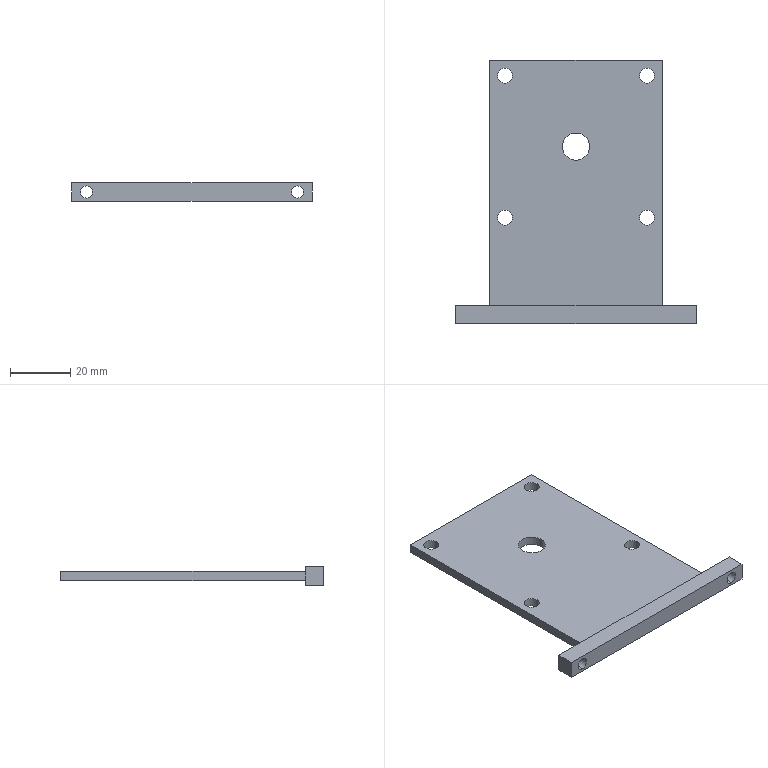Part | STEP file | Motor mounting plate | 1 solid | 29 faces | box 80 x 87.326 x 6 mm | volume 16246 mm3 | cylinder 14 | plane 11 | cone 4 | commonest cylinder face diameters 5 x8 4 x4 9 x2
STEP:
#1=CARTESIAN_POINT('',(-35.,-52.776,-0.5));
#2=VERTEX_POINT('',#1);
#3=CARTESIAN_POINT('',(-35.,-52.776,3.5));
#4=VERTEX_POINT('',#3);
#5=CARTESIAN_POINT('',(-35.,-52.776,1.5));
#6=DIRECTION('',(0.,1.,0.));
#7=DIRECTION('',(0.,0.,1.));
#8=AXIS2_PLACEMENT_3D('',#5,#6,#7);
#9=CIRCLE('',#8,2.);
#10=EDGE_CURVE('',#2,#4,#9,.T.);
#11=ORIENTED_EDGE('',*,*,#10,.F.);
#12=CARTESIAN_POINT('',(-35.,-52.751,-0.525));
#13=VERTEX_POINT('',#12);
#14=CARTESIAN_POINT('',(-35.,-52.751,-0.525));
#15=DIRECTION('',(0.,0.7071,-0.7071));
#16=VECTOR('',#15,1000.);
#17=LINE('',#14,#16);
#18=EDGE_CURVE('',#2,#13,#17,.T.);
#19=ORIENTED_EDGE('',*,*,#18,.T.);
#20=CARTESIAN_POINT('',(-35.,-52.751,3.525));
#21=VERTEX_POINT('',#20);
#22=CARTESIAN_POINT('',(-35.,-52.751,1.5));
#23=DIRECTION('',(0.,1.,0.));
#24=DIRECTION('',(0.,0.,1.));
#25=AXIS2_PLACEMENT_3D('',#22,#23,#24);
#26=CIRCLE('',#25,2.025);
#27=EDGE_CURVE('',#13,#21,#26,.T.);
#28=ORIENTED_EDGE('',*,*,#27,.T.);
#29=CARTESIAN_POINT('',(-35.,-52.751,3.525));
#30=DIRECTION('',(0.,0.7071,0.7071));
#31=VECTOR('',#30,1000.);
#32=LINE('',#29,#31);
#33=EDGE_CURVE('',#4,#21,#32,.T.);
#34=ORIENTED_EDGE('',*,*,#33,.F.);
#35=EDGE_LOOP('',(#11,#19,#28,#34));
#36=FACE_OUTER_BOUND('',#35,.T.);
#37=CARTESIAN_POINT('',(-35.,-52.751,1.5));
#38=DIRECTION('',(0.,1.,0.));
#39=DIRECTION('',(0.,0.,1.));
#40=AXIS2_PLACEMENT_3D('',#37,#38,#39);
#41=CONICAL_SURFACE('',#40,2.025,0.7854);
#42=ADVANCED_FACE('',(#36),#41,.F.);
#43=CARTESIAN_POINT('',(-35.,-58.751,3.5));
#44=VERTEX_POINT('',#43);
#45=CARTESIAN_POINT('',(-35.,-58.751,-0.5));
#46=VERTEX_POINT('',#45);
#47=CARTESIAN_POINT('',(-35.,-58.751,1.5));
#48=DIRECTION('',(0.,-1.,0.));
#49=DIRECTION('',(0.,0.,-1.));
#50=AXIS2_PLACEMENT_3D('',#47,#48,#49);
#51=CIRCLE('',#50,2.);
#52=EDGE_CURVE('',#44,#46,#51,.T.);
#53=ORIENTED_EDGE('',*,*,#52,.T.);
#54=CARTESIAN_POINT('',(-35.,-52.751,-0.5));
#55=DIRECTION('',(0.,1.,0.));
#56=VECTOR('',#55,1000.);
#57=LINE('',#54,#56);
#58=EDGE_CURVE('',#46,#2,#57,.T.);
#59=ORIENTED_EDGE('',*,*,#58,.T.);
#60=ORIENTED_EDGE('',*,*,#10,.T.);
#61=CARTESIAN_POINT('',(-35.,-52.751,3.5));
#62=DIRECTION('',(0.,1.,0.));
#63=VECTOR('',#62,1000.);
#64=LINE('',#61,#63);
#65=EDGE_CURVE('',#44,#4,#64,.T.);
#66=ORIENTED_EDGE('',*,*,#65,.F.);
#67=EDGE_LOOP('',(#53,#59,#60,#66));
#68=FACE_OUTER_BOUND('',#67,.T.);
#69=CARTESIAN_POINT('',(-35.,-52.751,1.5));
#70=DIRECTION('',(0.,1.,0.));
#71=DIRECTION('',(0.,0.,1.));
#72=AXIS2_PLACEMENT_3D('',#69,#70,#71);
#73=CYLINDRICAL_SURFACE('',#72,2.);
#74=ADVANCED_FACE('',(#68),#73,.F.);
#75=CARTESIAN_POINT('',(35.,-52.776,-0.5));
#76=VERTEX_POINT('',#75);
#77=CARTESIAN_POINT('',(35.,-52.776,3.5));
#78=VERTEX_POINT('',#77);
#79=CARTESIAN_POINT('',(35.,-52.776,1.5));
#80=DIRECTION('',(0.,1.,0.));
#81=DIRECTION('',(0.,0.,1.));
#82=AXIS2_PLACEMENT_3D('',#79,#80,#81);
#83=CIRCLE('',#82,2.);
#84=EDGE_CURVE('',#76,#78,#83,.T.);
#85=ORIENTED_EDGE('',*,*,#84,.F.);
#86=CARTESIAN_POINT('',(35.,-52.751,-0.525));
#87=VERTEX_POINT('',#86);
#88=CARTESIAN_POINT('',(35.,-52.751,-0.525));
#89=DIRECTION('',(0.,0.7071,-0.7071));
#90=VECTOR('',#89,1000.);
#91=LINE('',#88,#90);
#92=EDGE_CURVE('',#76,#87,#91,.T.);
#93=ORIENTED_EDGE('',*,*,#92,.T.);
#94=CARTESIAN_POINT('',(35.,-52.751,3.525));
#95=VERTEX_POINT('',#94);
#96=CARTESIAN_POINT('',(35.,-52.751,1.5));
#97=DIRECTION('',(0.,1.,0.));
#98=DIRECTION('',(0.,0.,1.));
#99=AXIS2_PLACEMENT_3D('',#96,#97,#98);
#100=CIRCLE('',#99,2.025);
#101=EDGE_CURVE('',#87,#95,#100,.T.);
#102=ORIENTED_EDGE('',*,*,#101,.T.);
#103=CARTESIAN_POINT('',(35.,-52.751,3.525));
#104=DIRECTION('',(0.,0.7071,0.7071));
#105=VECTOR('',#104,1000.);
#106=LINE('',#103,#105);
#107=EDGE_CURVE('',#78,#95,#106,.T.);
#108=ORIENTED_EDGE('',*,*,#107,.F.);
#109=EDGE_LOOP('',(#85,#93,#102,#108));
#110=FACE_OUTER_BOUND('',#109,.T.);
#111=CARTESIAN_POINT('',(35.,-52.751,1.5));
#112=DIRECTION('',(0.,1.,0.));
#113=DIRECTION('',(0.,0.,1.));
#114=AXIS2_PLACEMENT_3D('',#111,#112,#113);
#115=CONICAL_SURFACE('',#114,2.025,0.7854);
#116=ADVANCED_FACE('',(#110),#115,.F.);
#117=CARTESIAN_POINT('',(35.,-58.751,3.5));
#118=VERTEX_POINT('',#117);
#119=CARTESIAN_POINT('',(35.,-58.751,-0.5));
#120=VERTEX_POINT('',#119);
#121=CARTESIAN_POINT('',(35.,-58.751,1.5));
#122=DIRECTION('',(0.,-1.,0.));
#123=DIRECTION('',(0.,0.,-1.));
#124=AXIS2_PLACEMENT_3D('',#121,#122,#123);
#125=CIRCLE('',#124,2.);
#126=EDGE_CURVE('',#118,#120,#125,.T.);
#127=ORIENTED_EDGE('',*,*,#126,.T.);
#128=CARTESIAN_POINT('',(35.,-52.751,-0.5));
#129=DIRECTION('',(0.,1.,0.));
#130=VECTOR('',#129,1000.);
#131=LINE('',#128,#130);
#132=EDGE_CURVE('',#120,#76,#131,.T.);
#133=ORIENTED_EDGE('',*,*,#132,.T.);
#134=ORIENTED_EDGE('',*,*,#84,.T.);
#135=CARTESIAN_POINT('',(35.,-52.751,3.5));
#136=DIRECTION('',(0.,1.,0.));
#137=VECTOR('',#136,1000.);
#138=LINE('',#135,#137);
#139=EDGE_CURVE('',#118,#78,#138,.T.);
#140=ORIENTED_EDGE('',*,*,#139,.F.);
#141=EDGE_LOOP('',(#127,#133,#134,#140));
#142=FACE_OUTER_BOUND('',#141,.T.);
#143=CARTESIAN_POINT('',(35.,-52.751,1.5));
#144=DIRECTION('',(0.,1.,0.));
#145=DIRECTION('',(0.,0.,1.));
#146=AXIS2_PLACEMENT_3D('',#143,#144,#145);
#147=CYLINDRICAL_SURFACE('',#146,2.);
#148=ADVANCED_FACE('',(#142),#147,.F.);
#149=CARTESIAN_POINT('',(26.07,-23.57,0.));
#150=VERTEX_POINT('',#149);
#151=CARTESIAN_POINT('',(21.07,-23.57,0.));
#152=VERTEX_POINT('',#151);
#153=CARTESIAN_POINT('',(23.57,-23.57,0.));
#154=DIRECTION('',(0.,0.,-1.));
#155=DIRECTION('',(1.,0.,0.));
#156=AXIS2_PLACEMENT_3D('',#153,#154,#155);
#157=CIRCLE('',#156,2.5);
#158=EDGE_CURVE('',#150,#152,#157,.T.);
#159=ORIENTED_EDGE('',*,*,#158,.T.);
#160=CARTESIAN_POINT('',(21.07,-23.57,3.));
#161=VERTEX_POINT('',#160);
#162=CARTESIAN_POINT('',(21.07,-23.57,-0.001));
#163=DIRECTION('',(0.,0.,1.));
#164=VECTOR('',#163,1000.);
#165=LINE('',#162,#164);
#166=EDGE_CURVE('',#152,#161,#165,.T.);
#167=ORIENTED_EDGE('',*,*,#166,.T.);
#168=CARTESIAN_POINT('',(26.07,-23.57,3.));
#169=VERTEX_POINT('',#168);
#170=CARTESIAN_POINT('',(23.57,-23.57,3.));
#171=DIRECTION('',(0.,0.,1.));
#172=DIRECTION('',(1.,0.,0.));
#173=AXIS2_PLACEMENT_3D('',#170,#171,#172);
#174=CIRCLE('',#173,2.5);
#175=EDGE_CURVE('',#161,#169,#174,.T.);
#176=ORIENTED_EDGE('',*,*,#175,.T.);
#177=CARTESIAN_POINT('',(26.07,-23.57,-0.001));
#178=DIRECTION('',(0.,0.,1.));
#179=VECTOR('',#178,1000.);
#180=LINE('',#177,#179);
#181=EDGE_CURVE('',#150,#169,#180,.T.);
#182=ORIENTED_EDGE('',*,*,#181,.F.);
#183=EDGE_LOOP('',(#159,#167,#176,#182));
#184=FACE_OUTER_BOUND('',#183,.T.);
#185=CARTESIAN_POINT('',(23.57,-23.57,-0.001));
#186=DIRECTION('',(0.,0.,1.));
#187=DIRECTION('',(1.,0.,0.));
#188=AXIS2_PLACEMENT_3D('',#185,#186,#187);
#189=CYLINDRICAL_SURFACE('',#188,2.5);
#190=ADVANCED_FACE('',(#184),#189,.F.);
#191=CARTESIAN_POINT('',(-21.07,-23.57,0.));
#192=VERTEX_POINT('',#191);
#193=CARTESIAN_POINT('',(-26.07,-23.57,0.));
#194=VERTEX_POINT('',#193);
#195=CARTESIAN_POINT('',(-23.57,-23.57,0.));
#196=DIRECTION('',(0.,0.,-1.));
#197=DIRECTION('',(1.,0.,0.));
#198=AXIS2_PLACEMENT_3D('',#195,#196,#197);
#199=CIRCLE('',#198,2.5);
#200=EDGE_CURVE('',#192,#194,#199,.T.);
#201=ORIENTED_EDGE('',*,*,#200,.T.);
#202=CARTESIAN_POINT('',(-26.07,-23.57,3.));
#203=VERTEX_POINT('',#202);
#204=CARTESIAN_POINT('',(-26.07,-23.57,-0.001));
#205=DIRECTION('',(0.,0.,1.));
#206=VECTOR('',#205,1000.);
#207=LINE('',#204,#206);
#208=EDGE_CURVE('',#194,#203,#207,.T.);
#209=ORIENTED_EDGE('',*,*,#208,.T.);
#210=CARTESIAN_POINT('',(-21.07,-23.57,3.));
#211=VERTEX_POINT('',#210);
#212=CARTESIAN_POINT('',(-23.57,-23.57,3.));
#213=DIRECTION('',(0.,0.,1.));
#214=DIRECTION('',(1.,0.,0.));
#215=AXIS2_PLACEMENT_3D('',#212,#213,#214);
#216=CIRCLE('',#215,2.5);
#217=EDGE_CURVE('',#203,#211,#216,.T.);
#218=ORIENTED_EDGE('',*,*,#217,.T.);
#219=CARTESIAN_POINT('',(-21.07,-23.57,-0.001));
#220=DIRECTION('',(0.,0.,1.));
#221=VECTOR('',#220,1000.);
#222=LINE('',#219,#221);
#223=EDGE_CURVE('',#192,#211,#222,.T.);
#224=ORIENTED_EDGE('',*,*,#223,.F.);
#225=EDGE_LOOP('',(#201,#209,#218,#224));
#226=FACE_OUTER_BOUND('',#225,.T.);
#227=CARTESIAN_POINT('',(-23.57,-23.57,-0.001));
#228=DIRECTION('',(0.,0.,1.));
#229=DIRECTION('',(1.,0.,0.));
#230=AXIS2_PLACEMENT_3D('',#227,#228,#229);
#231=CYLINDRICAL_SURFACE('',#230,2.5);
#232=ADVANCED_FACE('',(#226),#231,.F.);
#233=CARTESIAN_POINT('',(-21.07,23.57,0.));
#234=VERTEX_POINT('',#233);
#235=CARTESIAN_POINT('',(-26.07,23.57,0.));
#236=VERTEX_POINT('',#235);
#237=CARTESIAN_POINT('',(-23.57,23.57,0.));
#238=DIRECTION('',(0.,0.,-1.));
#239=DIRECTION('',(1.,0.,0.));
#240=AXIS2_PLACEMENT_3D('',#237,#238,#239);
#241=CIRCLE('',#240,2.5);
#242=EDGE_CURVE('',#234,#236,#241,.T.);
#243=ORIENTED_EDGE('',*,*,#242,.T.);
#244=CARTESIAN_POINT('',(-26.07,23.57,3.));
#245=VERTEX_POINT('',#244);
#246=CARTESIAN_POINT('',(-26.07,23.57,-0.001));
#247=DIRECTION('',(0.,0.,1.));
#248=VECTOR('',#247,1000.);
#249=LINE('',#246,#248);
#250=EDGE_CURVE('',#236,#245,#249,.T.);
#251=ORIENTED_EDGE('',*,*,#250,.T.);
#252=CARTESIAN_POINT('',(-21.07,23.57,3.));
#253=VERTEX_POINT('',#252);
#254=CARTESIAN_POINT('',(-23.57,23.57,3.));
#255=DIRECTION('',(0.,0.,1.));
#256=DIRECTION('',(1.,0.,0.));
#257=AXIS2_PLACEMENT_3D('',#254,#255,#256);
#258=CIRCLE('',#257,2.5);
#259=EDGE_CURVE('',#245,#253,#258,.T.);
#260=ORIENTED_EDGE('',*,*,#259,.T.);
#261=CARTESIAN_POINT('',(-21.07,23.57,-0.001));
#262=DIRECTION('',(0.,0.,1.));
#263=VECTOR('',#262,1000.);
#264=LINE('',#261,#263);
#265=EDGE_CURVE('',#234,#253,#264,.T.);
#266=ORIENTED_EDGE('',*,*,#265,.F.);
#267=EDGE_LOOP('',(#243,#251,#260,#266));
#268=FACE_OUTER_BOUND('',#267,.T.);
#269=CARTESIAN_POINT('',(-23.57,23.57,-0.001));
#270=DIRECTION('',(0.,0.,1.));
#271=DIRECTION('',(1.,0.,0.));
#272=AXIS2_PLACEMENT_3D('',#269,#270,#271);
#273=CYLINDRICAL_SURFACE('',#272,2.5);
#274=ADVANCED_FACE('',(#268),#273,.F.);
#275=CARTESIAN_POINT('',(26.07,23.57,0.));
#276=VERTEX_POINT('',#275);
#277=CARTESIAN_POINT('',(21.07,23.57,0.));
#278=VERTEX_POINT('',#277);
#279=CARTESIAN_POINT('',(23.57,23.57,0.));
#280=DIRECTION('',(0.,0.,-1.));
#281=DIRECTION('',(1.,0.,0.));
#282=AXIS2_PLACEMENT_3D('',#279,#280,#281);
#283=CIRCLE('',#282,2.5);
#284=EDGE_CURVE('',#276,#278,#283,.T.);
#285=ORIENTED_EDGE('',*,*,#284,.T.);
#286=CARTESIAN_POINT('',(21.07,23.57,3.));
#287=VERTEX_POINT('',#286);
#288=CARTESIAN_POINT('',(21.07,23.57,-0.001));
#289=DIRECTION('',(0.,0.,1.));
#290=VECTOR('',#289,1000.);
#291=LINE('',#288,#290);
#292=EDGE_CURVE('',#278,#287,#291,.T.);
#293=ORIENTED_EDGE('',*,*,#292,.T.);
#294=CARTESIAN_POINT('',(26.07,23.57,3.));
#295=VERTEX_POINT('',#294);
#296=CARTESIAN_POINT('',(23.57,23.57,3.));
#297=DIRECTION('',(0.,0.,1.));
#298=DIRECTION('',(1.,0.,0.));
#299=AXIS2_PLACEMENT_3D('',#296,#297,#298);
#300=CIRCLE('',#299,2.5);
#301=EDGE_CURVE('',#287,#295,#300,.T.);
#302=ORIENTED_EDGE('',*,*,#301,.T.);
#303=CARTESIAN_POINT('',(26.07,23.57,-0.001));
#304=DIRECTION('',(0.,0.,1.));
#305=VECTOR('',#304,1000.);
#306=LINE('',#303,#305);
#307=EDGE_CURVE('',#276,#295,#306,.T.);
#308=ORIENTED_EDGE('',*,*,#307,.F.);
#309=EDGE_LOOP('',(#285,#293,#302,#308));
#310=FACE_OUTER_BOUND('',#309,.T.);
#311=CARTESIAN_POINT('',(23.57,23.57,-0.001));
#312=DIRECTION('',(0.,0.,1.));
#313=DIRECTION('',(1.,0.,0.));
#314=AXIS2_PLACEMENT_3D('',#311,#312,#313);
#315=CYLINDRICAL_SURFACE('',#314,2.5);
#316=ADVANCED_FACE('',(#310),#315,.F.);
#317=CARTESIAN_POINT('',(4.5,0.,0.));
#318=VERTEX_POINT('',#317);
#319=CARTESIAN_POINT('',(-4.5,0.,0.));
#320=VERTEX_POINT('',#319);
#321=CARTESIAN_POINT('',(0.,0.,0.));
#322=DIRECTION('',(0.,0.,-1.));
#323=DIRECTION('',(1.,0.,0.));
#324=AXIS2_PLACEMENT_3D('',#321,#322,#323);
#325=CIRCLE('',#324,4.5);
#326=EDGE_CURVE('',#318,#320,#325,.T.);
#327=ORIENTED_EDGE('',*,*,#326,.T.);
#328=CARTESIAN_POINT('',(-4.5,0.,3.));
#329=VERTEX_POINT('',#328);
#330=CARTESIAN_POINT('',(-4.5,0.,-0.001));
#331=DIRECTION('',(0.,0.,1.));
#332=VECTOR('',#331,1000.);
#333=LINE('',#330,#332);
#334=EDGE_CURVE('',#320,#329,#333,.T.);
#335=ORIENTED_EDGE('',*,*,#334,.T.);
#336=CARTESIAN_POINT('',(4.5,0.,3.));
#337=VERTEX_POINT('',#336);
#338=CARTESIAN_POINT('',(0.,0.,3.));
#339=DIRECTION('',(0.,0.,1.));
#340=DIRECTION('',(1.,0.,0.));
#341=AXIS2_PLACEMENT_3D('',#338,#339,#340);
#342=CIRCLE('',#341,4.5);
#343=EDGE_CURVE('',#329,#337,#342,.T.);
#344=ORIENTED_EDGE('',*,*,#343,.T.);
#345=CARTESIAN_POINT('',(4.5,0.,-0.001));
#346=DIRECTION('',(0.,0.,1.));
#347=VECTOR('',#346,1000.);
#348=LINE('',#345,#347);
#349=EDGE_CURVE('',#318,#337,#348,.T.);
#350=ORIENTED_EDGE('',*,*,#349,.F.);
#351=EDGE_LOOP('',(#327,#335,#344,#350));
#352=FACE_OUTER_BOUND('',#351,.T.);
#353=CARTESIAN_POINT('',(0.,0.,-0.001));
#354=DIRECTION('',(0.,0.,1.));
#355=DIRECTION('',(1.,0.,0.));
#356=AXIS2_PLACEMENT_3D('',#353,#354,#355);
#357=CYLINDRICAL_SURFACE('',#356,4.5);
#358=ADVANCED_FACE('',(#352),#357,.F.);
#359=CARTESIAN_POINT('',(-40.,-52.751,4.5));
#360=VERTEX_POINT('',#359);
#361=CARTESIAN_POINT('',(-40.,-52.751,-1.5));
#362=VERTEX_POINT('',#361);
#363=CARTESIAN_POINT('',(-40.,-52.751,3.));
#364=DIRECTION('',(0.,0.,-1.));
#365=VECTOR('',#364,1000.);
#366=LINE('',#363,#365);
#367=EDGE_CURVE('',#360,#362,#366,.T.);
#368=ORIENTED_EDGE('',*,*,#367,.F.);
#369=CARTESIAN_POINT('',(40.,-52.751,4.5));
#370=VERTEX_POINT('',#369);
#371=CARTESIAN_POINT('',(-40.,-52.751,4.5));
#372=DIRECTION('',(-1.,0.,0.));
#373=VECTOR('',#372,1000.);
#374=LINE('',#371,#373);
#375=EDGE_CURVE('',#370,#360,#374,.T.);
#376=ORIENTED_EDGE('',*,*,#375,.F.);
#377=CARTESIAN_POINT('',(40.,-52.751,-1.5));
#378=VERTEX_POINT('',#377);
#379=CARTESIAN_POINT('',(40.,-52.751,3.));
#380=DIRECTION('',(0.,0.,-1.));
#381=VECTOR('',#380,1000.);
#382=LINE('',#379,#381);
#383=EDGE_CURVE('',#370,#378,#382,.T.);
#384=ORIENTED_EDGE('',*,*,#383,.T.);
#385=CARTESIAN_POINT('',(-40.,-52.751,-1.5));
#386=DIRECTION('',(-1.,0.,0.));
#387=VECTOR('',#386,1000.);
#388=LINE('',#385,#387);
#389=EDGE_CURVE('',#378,#362,#388,.T.);
#390=ORIENTED_EDGE('',*,*,#389,.T.);
#391=EDGE_LOOP('',(#368,#376,#384,#390));
#392=FACE_OUTER_BOUND('',#391,.T.);
#393=CARTESIAN_POINT('',(-28.575,-52.751,3.));
#394=VERTEX_POINT('',#393);
#395=CARTESIAN_POINT('',(28.575,-52.751,3.));
#396=VERTEX_POINT('',#395);
#397=CARTESIAN_POINT('',(0.,-52.751,3.));
#398=DIRECTION('',(1.,0.,0.));
#399=VECTOR('',#398,1000.);
#400=LINE('',#397,#399);
#401=EDGE_CURVE('',#394,#396,#400,.T.);
#402=ORIENTED_EDGE('',*,*,#401,.F.);
#403=CARTESIAN_POINT('',(-28.575,-52.751,0.));
#404=VERTEX_POINT('',#403);
#405=CARTESIAN_POINT('',(-28.575,-52.751,3.));
#406=DIRECTION('',(0.,0.,-1.));
#407=VECTOR('',#406,1000.);
#408=LINE('',#405,#407);
#409=EDGE_CURVE('',#394,#404,#408,.T.);
#410=ORIENTED_EDGE('',*,*,#409,.T.);
#411=CARTESIAN_POINT('',(28.575,-52.751,0.));
#412=VERTEX_POINT('',#411);
#413=CARTESIAN_POINT('',(0.,-52.751,0.));
#414=DIRECTION('',(1.,0.,0.));
#415=VECTOR('',#414,1000.);
#416=LINE('',#413,#415);
#417=EDGE_CURVE('',#404,#412,#416,.T.);
#418=ORIENTED_EDGE('',*,*,#417,.T.);
#419=CARTESIAN_POINT('',(28.575,-52.751,3.));
#420=DIRECTION('',(0.,0.,-1.));
#421=VECTOR('',#420,1000.);
#422=LINE('',#419,#421);
#423=EDGE_CURVE('',#396,#412,#422,.T.);
#424=ORIENTED_EDGE('',*,*,#423,.F.);
#425=EDGE_LOOP('',(#402,#410,#418,#424));
#426=FACE_BOUND('',#425,.T.);
#427=CARTESIAN_POINT('',(35.,-52.751,1.5));
#428=DIRECTION('',(0.,1.,0.));
#429=DIRECTION('',(0.,0.,1.));
#430=AXIS2_PLACEMENT_3D('',#427,#428,#429);
#431=CIRCLE('',#430,2.025);
#432=EDGE_CURVE('',#95,#87,#431,.T.);
#433=ORIENTED_EDGE('',*,*,#432,.F.);
#434=ORIENTED_EDGE('',*,*,#101,.F.);
#435=EDGE_LOOP('',(#433,#434));
#436=FACE_BOUND('',#435,.T.);
#437=CARTESIAN_POINT('',(-35.,-52.751,1.5));
#438=DIRECTION('',(0.,1.,0.));
#439=DIRECTION('',(0.,0.,1.));
#440=AXIS2_PLACEMENT_3D('',#437,#438,#439);
#441=CIRCLE('',#440,2.025);
#442=EDGE_CURVE('',#21,#13,#441,.T.);
#443=ORIENTED_EDGE('',*,*,#442,.F.);
#444=ORIENTED_EDGE('',*,*,#27,.F.);
#445=EDGE_LOOP('',(#443,#444));
#446=FACE_BOUND('',#445,.T.);
#447=CARTESIAN_POINT('',(0.,-52.751,3.));
#448=DIRECTION('',(0.,-1.,0.));
#449=DIRECTION('',(1.,0.,0.));
#450=AXIS2_PLACEMENT_3D('',#447,#448,#449);
#451=PLANE('',#450);
#452=ADVANCED_FACE('',(#392,#426,#436,#446),#451,.F.);
#453=CARTESIAN_POINT('',(23.57,-23.57,3.));
#454=DIRECTION('',(0.,0.,1.));
#455=DIRECTION('',(1.,0.,0.));
#456=AXIS2_PLACEMENT_3D('',#453,#454,#455);
#457=CIRCLE('',#456,2.5);
#458=EDGE_CURVE('',#169,#161,#457,.T.);
#459=ORIENTED_EDGE('',*,*,#458,.F.);
#460=ORIENTED_EDGE('',*,*,#175,.F.);
#461=EDGE_LOOP('',(#459,#460));
#462=FACE_BOUND('',#461,.T.);
#463=CARTESIAN_POINT('',(-23.57,-23.57,3.));
#464=DIRECTION('',(0.,0.,1.));
#465=DIRECTION('',(1.,0.,0.));
#466=AXIS2_PLACEMENT_3D('',#463,#464,#465);
#467=CIRCLE('',#466,2.5);
#468=EDGE_CURVE('',#211,#203,#467,.T.);
#469=ORIENTED_EDGE('',*,*,#468,.F.);
#470=ORIENTED_EDGE('',*,*,#217,.F.);
#471=EDGE_LOOP('',(#469,#470));
#472=FACE_BOUND('',#471,.T.);
#473=CARTESIAN_POINT('',(-23.57,23.57,3.));
#474=DIRECTION('',(0.,0.,1.));
#475=DIRECTION('',(1.,0.,0.));
#476=AXIS2_PLACEMENT_3D('',#473,#474,#475);
#477=CIRCLE('',#476,2.5);
#478=EDGE_CURVE('',#253,#245,#477,.T.);
#479=ORIENTED_EDGE('',*,*,#478,.F.);
#480=ORIENTED_EDGE('',*,*,#259,.F.);
#481=EDGE_LOOP('',(#479,#480));
#482=FACE_BOUND('',#481,.T.);
#483=CARTESIAN_POINT('',(23.57,23.57,3.));
#484=DIRECTION('',(0.,0.,1.));
#485=DIRECTION('',(1.,0.,0.));
#486=AXIS2_PLACEMENT_3D('',#483,#484,#485);
#487=CIRCLE('',#486,2.5);
#488=EDGE_CURVE('',#295,#287,#487,.T.);
#489=ORIENTED_EDGE('',*,*,#488,.F.);
#490=ORIENTED_EDGE('',*,*,#301,.F.);
#491=EDGE_LOOP('',(#489,#490));
#492=FACE_BOUND('',#491,.T.);
#493=CARTESIAN_POINT('',(0.,0.,3.));
#494=DIRECTION('',(0.,0.,1.));
#495=DIRECTION('',(1.,0.,0.));
#496=AXIS2_PLACEMENT_3D('',#493,#494,#495);
#497=CIRCLE('',#496,4.5);
#498=EDGE_CURVE('',#337,#329,#497,.T.);
#499=ORIENTED_EDGE('',*,*,#498,.F.);
#500=ORIENTED_EDGE('',*,*,#343,.F.);
#501=EDGE_LOOP('',(#499,#500));
#502=FACE_BOUND('',#501,.T.);
#503=CARTESIAN_POINT('',(-28.575,28.575,3.));
#504=VERTEX_POINT('',#503);
#505=CARTESIAN_POINT('',(-28.575,0.,3.));
#506=DIRECTION('',(0.,1.,0.));
#507=VECTOR('',#506,1000.);
#508=LINE('',#505,#507);
#509=EDGE_CURVE('',#394,#504,#508,.T.);
#510=ORIENTED_EDGE('',*,*,#509,.F.);
#511=ORIENTED_EDGE('',*,*,#401,.T.);
#512=CARTESIAN_POINT('',(28.575,28.575,3.));
#513=VERTEX_POINT('',#512);
#514=CARTESIAN_POINT('',(28.575,0.,3.));
#515=DIRECTION('',(0.,-1.,0.));
#516=VECTOR('',#515,1000.);
#517=LINE('',#514,#516);
#518=EDGE_CURVE('',#513,#396,#517,.T.);
#519=ORIENTED_EDGE('',*,*,#518,.F.);
#520=CARTESIAN_POINT('',(0.,28.575,3.));
#521=DIRECTION('',(-1.,0.,0.));
#522=VECTOR('',#521,1000.);
#523=LINE('',#520,#522);
#524=EDGE_CURVE('',#513,#504,#523,.T.);
#525=ORIENTED_EDGE('',*,*,#524,.T.);
#526=EDGE_LOOP('',(#510,#511,#519,#525));
#527=FACE_OUTER_BOUND('',#526,.T.);
#528=CARTESIAN_POINT('',(0.,0.,3.));
#529=DIRECTION('',(0.,0.,1.));
#530=DIRECTION('',(1.,0.,0.));
#531=AXIS2_PLACEMENT_3D('',#528,#529,#530);
#532=PLANE('',#531);
#533=ADVANCED_FACE('',(#462,#472,#482,#492,#502,#527),#532,.T.);
#534=ORIENTED_EDGE('',*,*,#326,.F.);
#535=CARTESIAN_POINT('',(0.,0.,0.));
#536=DIRECTION('',(0.,0.,-1.));
#537=DIRECTION('',(1.,0.,0.));
#538=AXIS2_PLACEMENT_3D('',#535,#536,#537);
#539=CIRCLE('',#538,4.5);
#540=EDGE_CURVE('',#320,#318,#539,.T.);
#541=ORIENTED_EDGE('',*,*,#540,.F.);
#542=EDGE_LOOP('',(#534,#541));
#543=FACE_BOUND('',#542,.T.);
#544=ORIENTED_EDGE('',*,*,#284,.F.);
#545=CARTESIAN_POINT('',(23.57,23.57,0.));
#546=DIRECTION('',(0.,0.,-1.));
#547=DIRECTION('',(1.,0.,0.));
#548=AXIS2_PLACEMENT_3D('',#545,#546,#547);
#549=CIRCLE('',#548,2.5);
#550=EDGE_CURVE('',#278,#276,#549,.T.);
#551=ORIENTED_EDGE('',*,*,#550,.F.);
#552=EDGE_LOOP('',(#544,#551));
#553=FACE_BOUND('',#552,.T.);
#554=ORIENTED_EDGE('',*,*,#242,.F.);
#555=CARTESIAN_POINT('',(-23.57,23.57,0.));
#556=DIRECTION('',(0.,0.,-1.));
#557=DIRECTION('',(1.,0.,0.));
#558=AXIS2_PLACEMENT_3D('',#555,#556,#557);
#559=CIRCLE('',#558,2.5);
#560=EDGE_CURVE('',#236,#234,#559,.T.);
#561=ORIENTED_EDGE('',*,*,#560,.F.);
#562=EDGE_LOOP('',(#554,#561));
#563=FACE_BOUND('',#562,.T.);
#564=ORIENTED_EDGE('',*,*,#200,.F.);
#565=CARTESIAN_POINT('',(-23.57,-23.57,0.));
#566=DIRECTION('',(0.,0.,-1.));
#567=DIRECTION('',(1.,0.,0.));
#568=AXIS2_PLACEMENT_3D('',#565,#566,#567);
#569=CIRCLE('',#568,2.5);
#570=EDGE_CURVE('',#194,#192,#569,.T.);
#571=ORIENTED_EDGE('',*,*,#570,.F.);
#572=EDGE_LOOP('',(#564,#571));
#573=FACE_BOUND('',#572,.T.);
#574=ORIENTED_EDGE('',*,*,#158,.F.);
#575=CARTESIAN_POINT('',(23.57,-23.57,0.));
#576=DIRECTION('',(0.,0.,-1.));
#577=DIRECTION('',(1.,0.,0.));
#578=AXIS2_PLACEMENT_3D('',#575,#576,#577);
#579=CIRCLE('',#578,2.5);
#580=EDGE_CURVE('',#152,#150,#579,.T.);
#581=ORIENTED_EDGE('',*,*,#580,.F.);
#582=EDGE_LOOP('',(#574,#581));
#583=FACE_BOUND('',#582,.T.);
#584=ORIENTED_EDGE('',*,*,#417,.F.);
#585=CARTESIAN_POINT('',(-28.575,28.575,0.));
#586=VERTEX_POINT('',#585);
#587=CARTESIAN_POINT('',(-28.575,0.,0.));
#588=DIRECTION('',(0.,1.,0.));
#589=VECTOR('',#588,1000.);
#590=LINE('',#587,#589);
#591=EDGE_CURVE('',#404,#586,#590,.T.);
#592=ORIENTED_EDGE('',*,*,#591,.T.);
#593=CARTESIAN_POINT('',(28.575,28.575,0.));
#594=VERTEX_POINT('',#593);
#595=CARTESIAN_POINT('',(0.,28.575,0.));
#596=DIRECTION('',(-1.,0.,0.));
#597=VECTOR('',#596,1000.);
#598=LINE('',#595,#597);
#599=EDGE_CURVE('',#594,#586,#598,.T.);
#600=ORIENTED_EDGE('',*,*,#599,.F.);
#601=CARTESIAN_POINT('',(28.575,0.,0.));
#602=DIRECTION('',(0.,-1.,0.));
#603=VECTOR('',#602,1000.);
#604=LINE('',#601,#603);
#605=EDGE_CURVE('',#594,#412,#604,.T.);
#606=ORIENTED_EDGE('',*,*,#605,.T.);
#607=EDGE_LOOP('',(#584,#592,#600,#606));
#608=FACE_OUTER_BOUND('',#607,.T.);
#609=CARTESIAN_POINT('',(0.,0.,0.));
#610=DIRECTION('',(0.,0.,1.));
#611=DIRECTION('',(1.,0.,0.));
#612=AXIS2_PLACEMENT_3D('',#609,#610,#611);
#613=PLANE('',#612);
#614=ADVANCED_FACE('',(#543,#553,#563,#573,#583,#608),#613,.F.);
#615=ORIENTED_EDGE('',*,*,#605,.F.);
#616=CARTESIAN_POINT('',(28.575,28.575,3.));
#617=DIRECTION('',(0.,0.,-1.));
#618=VECTOR('',#617,1000.);
#619=LINE('',#616,#618);
#620=EDGE_CURVE('',#513,#594,#619,.T.);
#621=ORIENTED_EDGE('',*,*,#620,.F.);
#622=ORIENTED_EDGE('',*,*,#518,.T.);
#623=ORIENTED_EDGE('',*,*,#423,.T.);
#624=EDGE_LOOP('',(#615,#621,#622,#623));
#625=FACE_OUTER_BOUND('',#624,.T.);
#626=CARTESIAN_POINT('',(28.575,0.,3.));
#627=DIRECTION('',(1.,0.,0.));
#628=DIRECTION('',(0.,1.,0.));
#629=AXIS2_PLACEMENT_3D('',#626,#627,#628);
#630=PLANE('',#629);
#631=ADVANCED_FACE('',(#625),#630,.T.);
#632=ORIENTED_EDGE('',*,*,#599,.T.);
#633=CARTESIAN_POINT('',(-28.575,28.575,3.));
#634=DIRECTION('',(0.,0.,-1.));
#635=VECTOR('',#634,1000.);
#636=LINE('',#633,#635);
#637=EDGE_CURVE('',#504,#586,#636,.T.);
#638=ORIENTED_EDGE('',*,*,#637,.F.);
#639=ORIENTED_EDGE('',*,*,#524,.F.);
#640=ORIENTED_EDGE('',*,*,#620,.T.);
#641=EDGE_LOOP('',(#632,#638,#639,#640));
#642=FACE_OUTER_BOUND('',#641,.T.);
#643=CARTESIAN_POINT('',(0.,28.575,3.));
#644=DIRECTION('',(0.,-1.,0.));
#645=DIRECTION('',(1.,0.,0.));
#646=AXIS2_PLACEMENT_3D('',#643,#644,#645);
#647=PLANE('',#646);
#648=ADVANCED_FACE('',(#642),#647,.F.);
#649=ORIENTED_EDGE('',*,*,#591,.F.);
#650=ORIENTED_EDGE('',*,*,#409,.F.);
#651=ORIENTED_EDGE('',*,*,#509,.T.);
#652=ORIENTED_EDGE('',*,*,#637,.T.);
#653=EDGE_LOOP('',(#649,#650,#651,#652));
#654=FACE_OUTER_BOUND('',#653,.T.);
#655=CARTESIAN_POINT('',(-28.575,0.,3.));
#656=DIRECTION('',(-1.,0.,0.));
#657=DIRECTION('',(0.,-1.,0.));
#658=AXIS2_PLACEMENT_3D('',#655,#656,#657);
#659=PLANE('',#658);
#660=ADVANCED_FACE('',(#654),#659,.T.);
#661=ORIENTED_EDGE('',*,*,#367,.T.);
#662=CARTESIAN_POINT('',(-40.,-58.751,-1.5));
#663=VERTEX_POINT('',#662);
#664=CARTESIAN_POINT('',(-40.,-52.751,-1.5));
#665=DIRECTION('',(0.,-1.,0.));
#666=VECTOR('',#665,1000.);
#667=LINE('',#664,#666);
#668=EDGE_CURVE('',#362,#663,#667,.T.);
#669=ORIENTED_EDGE('',*,*,#668,.T.);
#670=CARTESIAN_POINT('',(-40.,-58.751,4.5));
#671=VERTEX_POINT('',#670);
#672=CARTESIAN_POINT('',(-40.,-58.751,3.));
#673=DIRECTION('',(0.,0.,-1.));
#674=VECTOR('',#673,1000.);
#675=LINE('',#672,#674);
#676=EDGE_CURVE('',#671,#663,#675,.T.);
#677=ORIENTED_EDGE('',*,*,#676,.F.);
#678=CARTESIAN_POINT('',(-40.,-52.751,4.5));
#679=DIRECTION('',(0.,-1.,0.));
#680=VECTOR('',#679,1000.);
#681=LINE('',#678,#680);
#682=EDGE_CURVE('',#360,#671,#681,.T.);
#683=ORIENTED_EDGE('',*,*,#682,.F.);
#684=EDGE_LOOP('',(#661,#669,#677,#683));
#685=FACE_OUTER_BOUND('',#684,.T.);
#686=CARTESIAN_POINT('',(-40.,0.,3.));
#687=DIRECTION('',(1.,0.,0.));
#688=DIRECTION('',(0.,1.,0.));
#689=AXIS2_PLACEMENT_3D('',#686,#687,#688);
#690=PLANE('',#689);
#691=ADVANCED_FACE('',(#685),#690,.F.);
#692=ORIENTED_EDGE('',*,*,#52,.F.);
#693=CARTESIAN_POINT('',(-35.,-58.751,1.5));
#694=DIRECTION('',(0.,-1.,0.));
#695=DIRECTION('',(0.,0.,-1.));
#696=AXIS2_PLACEMENT_3D('',#693,#694,#695);
#697=CIRCLE('',#696,2.);
#698=EDGE_CURVE('',#46,#44,#697,.T.);
#699=ORIENTED_EDGE('',*,*,#698,.F.);
#700=EDGE_LOOP('',(#692,#699));
#701=FACE_BOUND('',#700,.T.);
#702=ORIENTED_EDGE('',*,*,#126,.F.);
#703=CARTESIAN_POINT('',(35.,-58.751,1.5));
#704=DIRECTION('',(0.,-1.,0.));
#705=DIRECTION('',(0.,0.,-1.));
#706=AXIS2_PLACEMENT_3D('',#703,#704,#705);
#707=CIRCLE('',#706,2.);
#708=EDGE_CURVE('',#120,#118,#707,.T.);
#709=ORIENTED_EDGE('',*,*,#708,.F.);
#710=EDGE_LOOP('',(#702,#709));
#711=FACE_BOUND('',#710,.T.);
#712=ORIENTED_EDGE('',*,*,#676,.T.);
#713=CARTESIAN_POINT('',(40.,-58.751,-1.5));
#714=VERTEX_POINT('',#713);
#715=CARTESIAN_POINT('',(-40.,-58.751,-1.5));
#716=DIRECTION('',(1.,0.,0.));
#717=VECTOR('',#716,1000.);
#718=LINE('',#715,#717);
#719=EDGE_CURVE('',#663,#714,#718,.T.);
#720=ORIENTED_EDGE('',*,*,#719,.T.);
#721=CARTESIAN_POINT('',(40.,-58.751,4.5));
#722=VERTEX_POINT('',#721);
#723=CARTESIAN_POINT('',(40.,-58.751,3.));
#724=DIRECTION('',(0.,0.,-1.));
#725=VECTOR('',#724,1000.);
#726=LINE('',#723,#725);
#727=EDGE_CURVE('',#722,#714,#726,.T.);
#728=ORIENTED_EDGE('',*,*,#727,.F.);
#729=CARTESIAN_POINT('',(-40.,-58.751,4.5));
#730=DIRECTION('',(1.,0.,0.));
#731=VECTOR('',#730,1000.);
#732=LINE('',#729,#731);
#733=EDGE_CURVE('',#671,#722,#732,.T.);
#734=ORIENTED_EDGE('',*,*,#733,.F.);
#735=EDGE_LOOP('',(#712,#720,#728,#734));
#736=FACE_OUTER_BOUND('',#735,.T.);
#737=CARTESIAN_POINT('',(0.,-58.751,3.));
#738=DIRECTION('',(0.,-1.,0.));
#739=DIRECTION('',(0.,0.,-1.));
#740=AXIS2_PLACEMENT_3D('',#737,#738,#739);
#741=PLANE('',#740);
#742=ADVANCED_FACE('',(#701,#711,#736),#741,.T.);
#743=ORIENTED_EDGE('',*,*,#727,.T.);
#744=CARTESIAN_POINT('',(40.,-52.751,-1.5));
#745=DIRECTION('',(0.,1.,0.));
#746=VECTOR('',#745,1000.);
#747=LINE('',#744,#746);
#748=EDGE_CURVE('',#714,#378,#747,.T.);
#749=ORIENTED_EDGE('',*,*,#748,.T.);
#750=ORIENTED_EDGE('',*,*,#383,.F.);
#751=CARTESIAN_POINT('',(40.,-52.751,4.5));
#752=DIRECTION('',(0.,1.,0.));
#753=VECTOR('',#752,1000.);
#754=LINE('',#751,#753);
#755=EDGE_CURVE('',#722,#370,#754,.T.);
#756=ORIENTED_EDGE('',*,*,#755,.F.);
#757=EDGE_LOOP('',(#743,#749,#750,#756));
#758=FACE_OUTER_BOUND('',#757,.T.);
#759=CARTESIAN_POINT('',(40.,0.,3.));
#760=DIRECTION('',(1.,0.,0.));
#761=DIRECTION('',(0.,1.,0.));
#762=AXIS2_PLACEMENT_3D('',#759,#760,#761);
#763=PLANE('',#762);
#764=ADVANCED_FACE('',(#758),#763,.T.);
#765=ORIENTED_EDGE('',*,*,#334,.F.);
#766=ORIENTED_EDGE('',*,*,#540,.T.);
#767=ORIENTED_EDGE('',*,*,#349,.T.);
#768=ORIENTED_EDGE('',*,*,#498,.T.);
#769=EDGE_LOOP('',(#765,#766,#767,#768));
#770=FACE_OUTER_BOUND('',#769,.T.);
#771=CARTESIAN_POINT('',(0.,0.,-0.001));
#772=DIRECTION('',(0.,0.,1.));
#773=DIRECTION('',(1.,0.,0.));
#774=AXIS2_PLACEMENT_3D('',#771,#772,#773);
#775=CYLINDRICAL_SURFACE('',#774,4.5);
#776=ADVANCED_FACE('',(#770),#775,.F.);
#777=ORIENTED_EDGE('',*,*,#292,.F.);
#778=ORIENTED_EDGE('',*,*,#550,.T.);
#779=ORIENTED_EDGE('',*,*,#307,.T.);
#780=ORIENTED_EDGE('',*,*,#488,.T.);
#781=EDGE_LOOP('',(#777,#778,#779,#780));
#782=FACE_OUTER_BOUND('',#781,.T.);
#783=CARTESIAN_POINT('',(23.57,23.57,-0.001));
#784=DIRECTION('',(0.,0.,1.));
#785=DIRECTION('',(1.,0.,0.));
#786=AXIS2_PLACEMENT_3D('',#783,#784,#785);
#787=CYLINDRICAL_SURFACE('',#786,2.5);
#788=ADVANCED_FACE('',(#782),#787,.F.);
#789=ORIENTED_EDGE('',*,*,#250,.F.);
#790=ORIENTED_EDGE('',*,*,#560,.T.);
#791=ORIENTED_EDGE('',*,*,#265,.T.);
#792=ORIENTED_EDGE('',*,*,#478,.T.);
#793=EDGE_LOOP('',(#789,#790,#791,#792));
#794=FACE_OUTER_BOUND('',#793,.T.);
#795=CARTESIAN_POINT('',(-23.57,23.57,-0.001));
#796=DIRECTION('',(0.,0.,1.));
#797=DIRECTION('',(1.,0.,0.));
#798=AXIS2_PLACEMENT_3D('',#795,#796,#797);
#799=CYLINDRICAL_SURFACE('',#798,2.5);
#800=ADVANCED_FACE('',(#794),#799,.F.);
#801=ORIENTED_EDGE('',*,*,#208,.F.);
#802=ORIENTED_EDGE('',*,*,#570,.T.);
#803=ORIENTED_EDGE('',*,*,#223,.T.);
#804=ORIENTED_EDGE('',*,*,#468,.T.);
#805=EDGE_LOOP('',(#801,#802,#803,#804));
#806=FACE_OUTER_BOUND('',#805,.T.);
#807=CARTESIAN_POINT('',(-23.57,-23.57,-0.001));
#808=DIRECTION('',(0.,0.,1.));
#809=DIRECTION('',(1.,0.,0.));
#810=AXIS2_PLACEMENT_3D('',#807,#808,#809);
#811=CYLINDRICAL_SURFACE('',#810,2.5);
#812=ADVANCED_FACE('',(#806),#811,.F.);
#813=ORIENTED_EDGE('',*,*,#166,.F.);
#814=ORIENTED_EDGE('',*,*,#580,.T.);
#815=ORIENTED_EDGE('',*,*,#181,.T.);
#816=ORIENTED_EDGE('',*,*,#458,.T.);
#817=EDGE_LOOP('',(#813,#814,#815,#816));
#818=FACE_OUTER_BOUND('',#817,.T.);
#819=CARTESIAN_POINT('',(23.57,-23.57,-0.001));
#820=DIRECTION('',(0.,0.,1.));
#821=DIRECTION('',(1.,0.,0.));
#822=AXIS2_PLACEMENT_3D('',#819,#820,#821);
#823=CYLINDRICAL_SURFACE('',#822,2.5);
#824=ADVANCED_FACE('',(#818),#823,.F.);
#825=ORIENTED_EDGE('',*,*,#668,.F.);
#826=ORIENTED_EDGE('',*,*,#389,.F.);
#827=ORIENTED_EDGE('',*,*,#748,.F.);
#828=ORIENTED_EDGE('',*,*,#719,.F.);
#829=EDGE_LOOP('',(#825,#826,#827,#828));
#830=FACE_OUTER_BOUND('',#829,.T.);
#831=CARTESIAN_POINT('',(0.,0.,-1.5));
#832=DIRECTION('',(0.,0.,1.));
#833=DIRECTION('',(1.,0.,0.));
#834=AXIS2_PLACEMENT_3D('',#831,#832,#833);
#835=PLANE('',#834);
#836=ADVANCED_FACE('',(#830),#835,.F.);
#837=ORIENTED_EDGE('',*,*,#682,.T.);
#838=ORIENTED_EDGE('',*,*,#733,.T.);
#839=ORIENTED_EDGE('',*,*,#755,.T.);
#840=ORIENTED_EDGE('',*,*,#375,.T.);
#841=EDGE_LOOP('',(#837,#838,#839,#840));
#842=FACE_OUTER_BOUND('',#841,.T.);
#843=CARTESIAN_POINT('',(0.,0.,4.5));
#844=DIRECTION('',(0.,0.,1.));
#845=DIRECTION('',(1.,0.,0.));
#846=AXIS2_PLACEMENT_3D('',#843,#844,#845);
#847=PLANE('',#846);
#848=ADVANCED_FACE('',(#842),#847,.T.);
#849=ORIENTED_EDGE('',*,*,#132,.F.);
#850=ORIENTED_EDGE('',*,*,#708,.T.);
#851=ORIENTED_EDGE('',*,*,#139,.T.);
#852=CARTESIAN_POINT('',(35.,-52.776,1.5));
#853=DIRECTION('',(0.,1.,0.));
#854=DIRECTION('',(0.,0.,1.));
#855=AXIS2_PLACEMENT_3D('',#852,#853,#854);
#856=CIRCLE('',#855,2.);
#857=EDGE_CURVE('',#78,#76,#856,.T.);
#858=ORIENTED_EDGE('',*,*,#857,.T.);
#859=EDGE_LOOP('',(#849,#850,#851,#858));
#860=FACE_OUTER_BOUND('',#859,.T.);
#861=CARTESIAN_POINT('',(35.,-52.751,1.5));
#862=DIRECTION('',(0.,1.,0.));
#863=DIRECTION('',(0.,0.,1.));
#864=AXIS2_PLACEMENT_3D('',#861,#862,#863);
#865=CYLINDRICAL_SURFACE('',#864,2.);
#866=ADVANCED_FACE('',(#860),#865,.F.);
#867=ORIENTED_EDGE('',*,*,#92,.F.);
#868=ORIENTED_EDGE('',*,*,#857,.F.);
#869=ORIENTED_EDGE('',*,*,#107,.T.);
#870=ORIENTED_EDGE('',*,*,#432,.T.);
#871=EDGE_LOOP('',(#867,#868,#869,#870));
#872=FACE_OUTER_BOUND('',#871,.T.);
#873=CARTESIAN_POINT('',(35.,-52.751,1.5));
#874=DIRECTION('',(0.,1.,0.));
#875=DIRECTION('',(0.,0.,1.));
#876=AXIS2_PLACEMENT_3D('',#873,#874,#875);
#877=CONICAL_SURFACE('',#876,2.025,0.7854);
#878=ADVANCED_FACE('',(#872),#877,.F.);
#879=ORIENTED_EDGE('',*,*,#58,.F.);
#880=ORIENTED_EDGE('',*,*,#698,.T.);
#881=ORIENTED_EDGE('',*,*,#65,.T.);
#882=CARTESIAN_POINT('',(-35.,-52.776,1.5));
#883=DIRECTION('',(0.,1.,0.));
#884=DIRECTION('',(0.,0.,1.));
#885=AXIS2_PLACEMENT_3D('',#882,#883,#884);
#886=CIRCLE('',#885,2.);
#887=EDGE_CURVE('',#4,#2,#886,.T.);
#888=ORIENTED_EDGE('',*,*,#887,.T.);
#889=EDGE_LOOP('',(#879,#880,#881,#888));
#890=FACE_OUTER_BOUND('',#889,.T.);
#891=CARTESIAN_POINT('',(-35.,-52.751,1.5));
#892=DIRECTION('',(0.,1.,0.));
#893=DIRECTION('',(0.,0.,1.));
#894=AXIS2_PLACEMENT_3D('',#891,#892,#893);
#895=CYLINDRICAL_SURFACE('',#894,2.);
#896=ADVANCED_FACE('',(#890),#895,.F.);
#897=ORIENTED_EDGE('',*,*,#18,.F.);
#898=ORIENTED_EDGE('',*,*,#887,.F.);
#899=ORIENTED_EDGE('',*,*,#33,.T.);
#900=ORIENTED_EDGE('',*,*,#442,.T.);
#901=EDGE_LOOP('',(#897,#898,#899,#900));
#902=FACE_OUTER_BOUND('',#901,.T.);
#903=CARTESIAN_POINT('',(-35.,-52.751,1.5));
#904=DIRECTION('',(0.,1.,0.));
#905=DIRECTION('',(0.,0.,1.));
#906=AXIS2_PLACEMENT_3D('',#903,#904,#905);
#907=CONICAL_SURFACE('',#906,2.025,0.7854);
#908=ADVANCED_FACE('',(#902),#907,.F.);
#909=CLOSED_SHELL('',(#42,#74,#116,#148,#190,#232,#274,#316,#358,#452,#533,#614,#631,#648,#660,#691,#742,#764,#776,#788,#800,#812,#824,#836,#848,#866,#878,#896,#908));
#910=MANIFOLD_SOLID_BREP('',#909);
#911=CARTESIAN_POINT('',(0.,0.,0.));
#912=DIRECTION('',(0.,0.,1.));
#913=DIRECTION('',(1.,0.,0.));
#914=AXIS2_PLACEMENT_3D('',#911,#912,#913);
#915=(LENGTH_UNIT()NAMED_UNIT(*)SI_UNIT(.MILLI.,.METRE.));
#916=UNCERTAINTY_MEASURE_WITH_UNIT(LENGTH_MEASURE(0.00001),#915,'','');
#917=(NAMED_UNIT(*)PLANE_ANGLE_UNIT()SI_UNIT($,.RADIAN.));
#918=(NAMED_UNIT(*)SI_UNIT($,.STERADIAN.)SOLID_ANGLE_UNIT());
#919=(GEOMETRIC_REPRESENTATION_CONTEXT(3)GLOBAL_UNCERTAINTY_ASSIGNED_CONTEXT((#916))GLOBAL_UNIT_ASSIGNED_CONTEXT((#915,#917,#918))REPRESENTATION_CONTEXT('',''));
#920=ADVANCED_BREP_SHAPE_REPRESENTATION('',(#910,#914),#919);